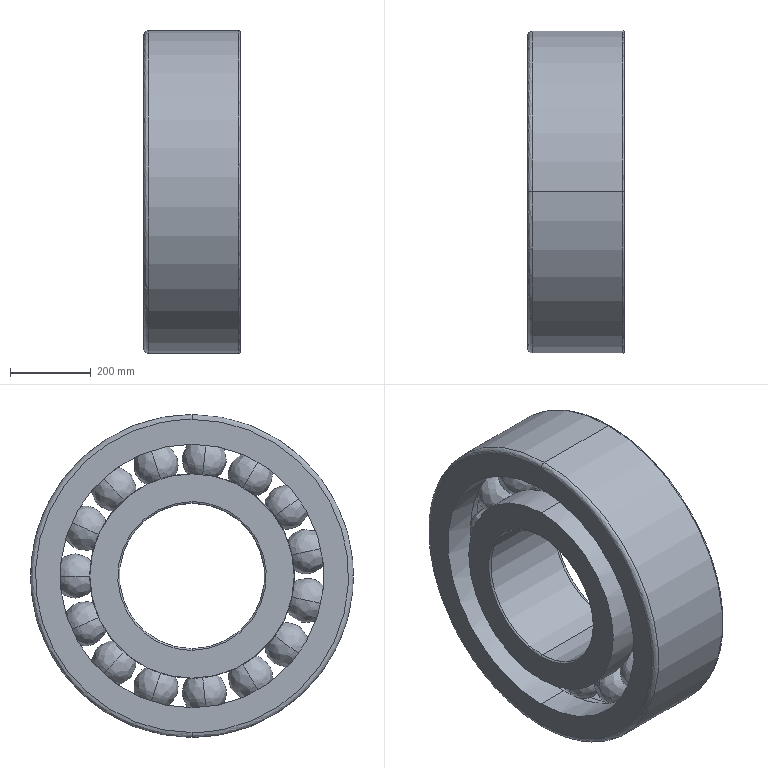Part | SolidWorks | features BaseBody 1, Scale 1 | 1 solid | 105 faces | box 240 x 800 x 800 mm | volume 68366602 mm3 | spline 86 | cylinder 14 | plane 5 | commonest cylinder face diameters 506.667 x4 360 x2 653.333 x2 672.933 x2 708.933 x2 800 x2